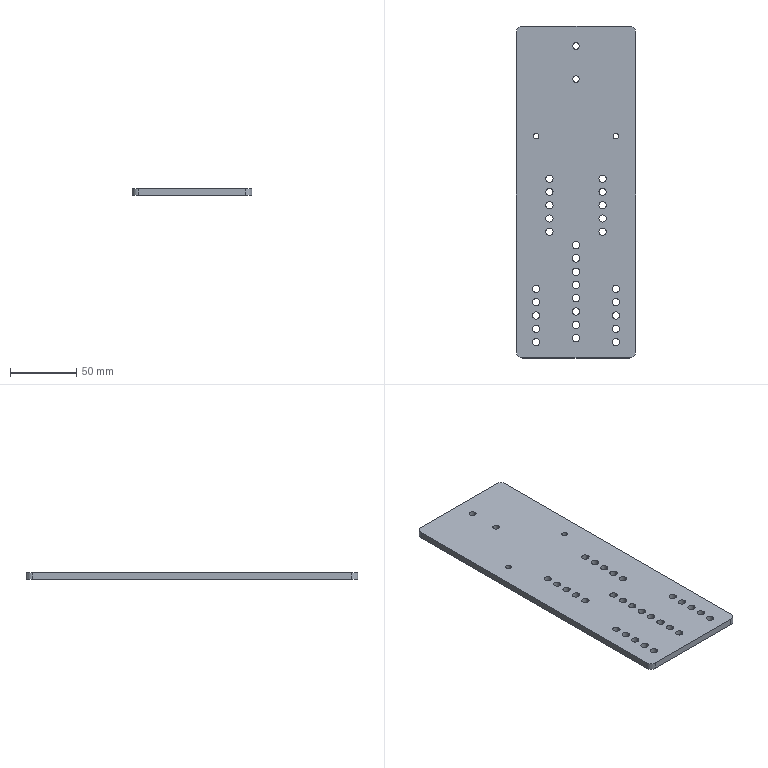Part | SolidWorks | features ICE 3, Extrusion 1, Fillet 1 | 1 solid | 74 faces | box 90 x 250 x 5 mm | volume 108732 mm3 | cylinder 68 | plane 6 | commonest cylinder face diameters 5.5 x56 4.2 x4 5 x4 10 x4